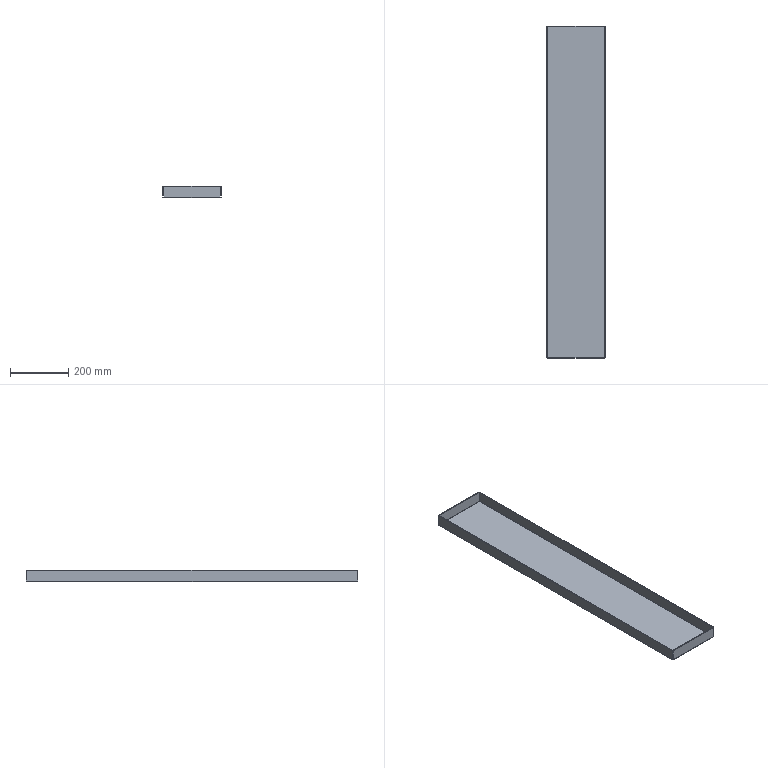Part | SolidWorks | features EdgeFlange 1, FlatPattern 1, SMBaseFlange 1, SheetMetal 1 | 1 solid | 38 faces | box 200 x 1140 x 40 mm | volume 654012 mm3 | plane 22 | spline 8 | cylinder 8 | commonest cylinder face diameters 1.473 x4 5.473 x4
STEP:
#1=CARTESIAN_POINT('',(97.263,567.263,-2.));
#2=VERTEX_POINT('',#1);
#3=CARTESIAN_POINT('',(97.263,-567.263,-2.));
#4=VERTEX_POINT('',#3);
#5=CARTESIAN_POINT('',(97.263,567.293,-2.));
#6=DIRECTION('',(0.,-1.,0.));
#7=VECTOR('',#6,1000.);
#8=LINE('',#5,#7);
#9=EDGE_CURVE('',#2,#4,#8,.T.);
#10=ORIENTED_EDGE('',*,*,#9,.T.);
#11=CARTESIAN_POINT('',(-97.263,-567.263,-2.));
#12=VERTEX_POINT('',#11);
#13=CARTESIAN_POINT('',(97.293,-567.263,-2.));
#14=DIRECTION('',(-1.,0.,0.));
#15=VECTOR('',#14,1000.);
#16=LINE('',#13,#15);
#17=EDGE_CURVE('',#4,#12,#16,.T.);
#18=ORIENTED_EDGE('',*,*,#17,.T.);
#19=CARTESIAN_POINT('',(-97.263,567.263,-2.));
#20=VERTEX_POINT('',#19);
#21=CARTESIAN_POINT('',(-97.263,-567.293,-2.));
#22=DIRECTION('',(0.,1.,0.));
#23=VECTOR('',#22,1000.);
#24=LINE('',#21,#23);
#25=EDGE_CURVE('',#12,#20,#24,.T.);
#26=ORIENTED_EDGE('',*,*,#25,.T.);
#27=CARTESIAN_POINT('',(-97.293,567.263,-2.));
#28=DIRECTION('',(1.,0.,0.));
#29=VECTOR('',#28,1000.);
#30=LINE('',#27,#29);
#31=EDGE_CURVE('',#20,#2,#30,.T.);
#32=ORIENTED_EDGE('',*,*,#31,.T.);
#33=EDGE_LOOP('',(#10,#18,#26,#32));
#34=FACE_OUTER_BOUND('',#33,.T.);
#35=CARTESIAN_POINT('',(0.,0.,-2.));
#36=DIRECTION('',(0.,0.,-1.));
#37=DIRECTION('',(-1.,0.,0.));
#38=AXIS2_PLACEMENT_3D('',#35,#36,#37);
#39=PLANE('',#38);
#40=ADVANCED_FACE('',(#34),#39,.T.);
#41=CARTESIAN_POINT('',(97.263,-567.263,0.));
#42=VERTEX_POINT('',#41);
#43=CARTESIAN_POINT('',(-97.263,-567.263,0.));
#44=VERTEX_POINT('',#43);
#45=CARTESIAN_POINT('',(97.293,-567.263,0.));
#46=DIRECTION('',(-1.,0.,0.));
#47=VECTOR('',#46,1000.);
#48=LINE('',#45,#47);
#49=EDGE_CURVE('',#42,#44,#48,.T.);
#50=ORIENTED_EDGE('',*,*,#49,.F.);
#51=CARTESIAN_POINT('',(97.263,567.263,0.));
#52=VERTEX_POINT('',#51);
#53=CARTESIAN_POINT('',(97.263,567.293,0.));
#54=DIRECTION('',(0.,-1.,0.));
#55=VECTOR('',#54,1000.);
#56=LINE('',#53,#55);
#57=EDGE_CURVE('',#52,#42,#56,.T.);
#58=ORIENTED_EDGE('',*,*,#57,.F.);
#59=CARTESIAN_POINT('',(-97.263,567.263,0.));
#60=VERTEX_POINT('',#59);
#61=CARTESIAN_POINT('',(-97.293,567.263,0.));
#62=DIRECTION('',(1.,0.,0.));
#63=VECTOR('',#62,1000.);
#64=LINE('',#61,#63);
#65=EDGE_CURVE('',#60,#52,#64,.T.);
#66=ORIENTED_EDGE('',*,*,#65,.F.);
#67=CARTESIAN_POINT('',(-97.263,-567.293,0.));
#68=DIRECTION('',(0.,1.,0.));
#69=VECTOR('',#68,1000.);
#70=LINE('',#67,#69);
#71=EDGE_CURVE('',#44,#60,#70,.T.);
#72=ORIENTED_EDGE('',*,*,#71,.F.);
#73=EDGE_LOOP('',(#50,#58,#66,#72));
#74=FACE_OUTER_BOUND('',#73,.T.);
#75=CARTESIAN_POINT('',(0.,0.,0.));
#76=DIRECTION('',(0.,0.,-1.));
#77=DIRECTION('',(-1.,0.,0.));
#78=AXIS2_PLACEMENT_3D('',#75,#76,#77);
#79=PLANE('',#78);
#80=ADVANCED_FACE('',(#74),#79,.F.);
#81=CARTESIAN_POINT('',(97.293,570.,0.7366));
#82=VERTEX_POINT('',#81);
#83=CARTESIAN_POINT('',(97.293,568.,0.7366));
#84=VERTEX_POINT('',#83);
#85=CARTESIAN_POINT('',(97.293,568.,0.7366));
#86=DIRECTION('',(0.,-1.,0.));
#87=VECTOR('',#86,1000.);
#88=LINE('',#85,#87);
#89=EDGE_CURVE('',#82,#84,#88,.T.);
#90=ORIENTED_EDGE('',*,*,#89,.T.);
#91=CARTESIAN_POINT('',(97.263,567.263,0.));
#92=CARTESIAN_POINT('',(97.268,567.456,0.));
#93=CARTESIAN_POINT('',(97.273,567.648,0.07939));
#94=CARTESIAN_POINT('',(97.283,567.921,0.3521));
#95=CARTESIAN_POINT('',(97.288,568.,0.5438));
#96=CARTESIAN_POINT('',(97.293,568.,0.7366));
#97=B_SPLINE_CURVE_WITH_KNOTS('',3,(#91,#92,#93,#94,#95,#96),.UNSPECIFIED.,.F.,.F.,(4,2,4),(0.,0.5,1.),.UNSPECIFIED.);
#98=EDGE_CURVE('',#52,#84,#97,.T.);
#99=ORIENTED_EDGE('',*,*,#98,.F.);
#100=CARTESIAN_POINT('',(97.263,567.263,0.));
#101=DIRECTION('',(0.,0.,-1.));
#102=VECTOR('',#101,1000.);
#103=LINE('',#100,#102);
#104=EDGE_CURVE('',#52,#2,#103,.T.);
#105=ORIENTED_EDGE('',*,*,#104,.T.);
#106=CARTESIAN_POINT('',(97.263,567.263,-2.));
#107=CARTESIAN_POINT('',(97.266,567.622,-2.));
#108=CARTESIAN_POINT('',(97.268,567.98,-1.929));
#109=CARTESIAN_POINT('',(97.273,568.642,-1.655));
#110=CARTESIAN_POINT('',(97.276,568.945,-1.452));
#111=CARTESIAN_POINT('',(97.281,569.452,-0.9452));
#112=CARTESIAN_POINT('',(97.283,569.655,-0.6416));
#113=CARTESIAN_POINT('',(97.288,569.929,0.0203));
#114=CARTESIAN_POINT('',(97.29,570.,0.3784));
#115=CARTESIAN_POINT('',(97.293,570.,0.7366));
#116=B_SPLINE_CURVE_WITH_KNOTS('',3,(#106,#107,#108,#109,#110,#111,#112,#113,#114,#115),.UNSPECIFIED.,.F.,.F.,(4,2,2,2,4),(0.,0.25,0.5,0.75,1.),.UNSPECIFIED.);
#117=EDGE_CURVE('',#2,#82,#116,.T.);
#118=ORIENTED_EDGE('',*,*,#117,.T.);
#119=EDGE_LOOP('',(#90,#99,#105,#118));
#120=FACE_OUTER_BOUND('',#119,.T.);
#121=CARTESIAN_POINT('',(97.263,567.263,-2.02));
#122=CARTESIAN_POINT('',(97.266,567.624,-2.02));
#123=CARTESIAN_POINT('',(97.268,567.985,-1.948));
#124=CARTESIAN_POINT('',(97.273,568.652,-1.672));
#125=CARTESIAN_POINT('',(97.276,568.957,-1.468));
#126=CARTESIAN_POINT('',(97.281,569.468,-0.9575));
#127=CARTESIAN_POINT('',(97.283,569.672,-0.6517));
#128=CARTESIAN_POINT('',(97.288,569.948,0.01507));
#129=CARTESIAN_POINT('',(97.29,570.02,0.3757));
#130=CARTESIAN_POINT('',(97.293,570.02,0.7366));
#131=CARTESIAN_POINT('',(97.263,567.263,-2.));
#132=CARTESIAN_POINT('',(97.266,567.622,-2.));
#133=CARTESIAN_POINT('',(97.268,567.98,-1.929));
#134=CARTESIAN_POINT('',(97.273,568.642,-1.655));
#135=CARTESIAN_POINT('',(97.276,568.945,-1.452));
#136=CARTESIAN_POINT('',(97.281,569.452,-0.9452));
#137=CARTESIAN_POINT('',(97.283,569.655,-0.6416));
#138=CARTESIAN_POINT('',(97.288,569.929,0.0203));
#139=CARTESIAN_POINT('',(97.29,570.,0.3783));
#140=CARTESIAN_POINT('',(97.293,570.,0.7366));
#141=CARTESIAN_POINT('',(97.263,567.263,0.));
#142=CARTESIAN_POINT('',(97.266,567.36,0.));
#143=CARTESIAN_POINT('',(97.268,567.456,0.01917));
#144=CARTESIAN_POINT('',(97.273,567.634,0.09297));
#145=CARTESIAN_POINT('',(97.276,567.716,0.1476));
#146=CARTESIAN_POINT('',(97.281,567.852,0.2839));
#147=CARTESIAN_POINT('',(97.283,567.907,0.3656));
#148=CARTESIAN_POINT('',(97.288,567.981,0.5438));
#149=CARTESIAN_POINT('',(97.29,568.,0.6402));
#150=CARTESIAN_POINT('',(97.293,568.,0.7366));
#151=CARTESIAN_POINT('',(97.263,567.263,0.0202));
#152=CARTESIAN_POINT('',(97.266,567.357,0.0202));
#153=CARTESIAN_POINT('',(97.268,567.451,0.03885));
#154=CARTESIAN_POINT('',(97.273,567.624,0.1106));
#155=CARTESIAN_POINT('',(97.276,567.704,0.1637));
#156=CARTESIAN_POINT('',(97.281,567.836,0.2963));
#157=CARTESIAN_POINT('',(97.283,567.889,0.3758));
#158=CARTESIAN_POINT('',(97.288,567.961,0.5491));
#159=CARTESIAN_POINT('',(97.29,567.98,0.6428));
#160=CARTESIAN_POINT('',(97.293,567.98,0.7366));
#161=B_SPLINE_SURFACE_WITH_KNOTS('',1,3,((#121,#122,#123,#124,#125,#126,#127,#128,#129,#130),(#131,#132,#133,#134,#135,#136,#137,#138,#139,#140),(#141,#142,#143,#144,#145,#146,#147,#148,#149,#150),(#151,#152,#153,#154,#155,#156,#157,#158,#159,#160)),.UNSPECIFIED.,.F.,.F.,.F.,(2,1,1,2),(4,2,2,2,4),(-0.01,0.,1.,1.01),(0.,0.25,0.5,0.75,1.),.UNSPECIFIED.);
#162=ADVANCED_FACE('',(#120),#161,.F.);
#163=CARTESIAN_POINT('',(-97.293,568.,0.7366));
#164=VERTEX_POINT('',#163);
#165=CARTESIAN_POINT('',(-97.293,568.,0.7366));
#166=CARTESIAN_POINT('',(-97.288,568.,0.5438));
#167=CARTESIAN_POINT('',(-97.283,567.921,0.3521));
#168=CARTESIAN_POINT('',(-97.273,567.648,0.07939));
#169=CARTESIAN_POINT('',(-97.268,567.456,0.));
#170=CARTESIAN_POINT('',(-97.263,567.263,0.));
#171=B_SPLINE_CURVE_WITH_KNOTS('',3,(#165,#166,#167,#168,#169,#170),.UNSPECIFIED.,.F.,.F.,(4,2,4),(0.,0.5,1.),.UNSPECIFIED.);
#172=EDGE_CURVE('',#164,#60,#171,.T.);
#173=ORIENTED_EDGE('',*,*,#172,.F.);
#174=CARTESIAN_POINT('',(-97.293,570.,0.7366));
#175=VERTEX_POINT('',#174);
#176=CARTESIAN_POINT('',(-97.293,568.,0.7366));
#177=DIRECTION('',(0.,-1.,0.));
#178=VECTOR('',#177,1000.);
#179=LINE('',#176,#178);
#180=EDGE_CURVE('',#175,#164,#179,.T.);
#181=ORIENTED_EDGE('',*,*,#180,.F.);
#182=CARTESIAN_POINT('',(-97.293,570.,0.7366));
#183=CARTESIAN_POINT('',(-97.29,570.,0.3784));
#184=CARTESIAN_POINT('',(-97.288,569.929,0.0203));
#185=CARTESIAN_POINT('',(-97.283,569.655,-0.6416));
#186=CARTESIAN_POINT('',(-97.281,569.452,-0.9452));
#187=CARTESIAN_POINT('',(-97.276,568.945,-1.452));
#188=CARTESIAN_POINT('',(-97.273,568.642,-1.655));
#189=CARTESIAN_POINT('',(-97.268,567.98,-1.929));
#190=CARTESIAN_POINT('',(-97.266,567.622,-2.));
#191=CARTESIAN_POINT('',(-97.263,567.263,-2.));
#192=B_SPLINE_CURVE_WITH_KNOTS('',3,(#182,#183,#184,#185,#186,#187,#188,#189,#190,#191),.UNSPECIFIED.,.F.,.F.,(4,2,2,2,4),(0.,0.25,0.5,0.75,1.),.UNSPECIFIED.);
#193=EDGE_CURVE('',#175,#20,#192,.T.);
#194=ORIENTED_EDGE('',*,*,#193,.T.);
#195=CARTESIAN_POINT('',(-97.263,567.263,0.));
#196=DIRECTION('',(0.,0.,-1.));
#197=VECTOR('',#196,1000.);
#198=LINE('',#195,#197);
#199=EDGE_CURVE('',#60,#20,#198,.T.);
#200=ORIENTED_EDGE('',*,*,#199,.F.);
#201=EDGE_LOOP('',(#173,#181,#194,#200));
#202=FACE_OUTER_BOUND('',#201,.T.);
#203=CARTESIAN_POINT('',(-97.293,570.02,0.7366));
#204=CARTESIAN_POINT('',(-97.29,570.02,0.3757));
#205=CARTESIAN_POINT('',(-97.288,569.948,0.01507));
#206=CARTESIAN_POINT('',(-97.283,569.672,-0.6517));
#207=CARTESIAN_POINT('',(-97.281,569.468,-0.9575));
#208=CARTESIAN_POINT('',(-97.276,568.957,-1.468));
#209=CARTESIAN_POINT('',(-97.273,568.652,-1.672));
#210=CARTESIAN_POINT('',(-97.268,567.985,-1.948));
#211=CARTESIAN_POINT('',(-97.266,567.624,-2.02));
#212=CARTESIAN_POINT('',(-97.263,567.263,-2.02));
#213=CARTESIAN_POINT('',(-97.293,570.,0.7366));
#214=CARTESIAN_POINT('',(-97.29,570.,0.3783));
#215=CARTESIAN_POINT('',(-97.288,569.929,0.0203));
#216=CARTESIAN_POINT('',(-97.283,569.655,-0.6416));
#217=CARTESIAN_POINT('',(-97.281,569.452,-0.9452));
#218=CARTESIAN_POINT('',(-97.276,568.945,-1.452));
#219=CARTESIAN_POINT('',(-97.273,568.642,-1.655));
#220=CARTESIAN_POINT('',(-97.268,567.98,-1.929));
#221=CARTESIAN_POINT('',(-97.266,567.622,-2.));
#222=CARTESIAN_POINT('',(-97.263,567.263,-2.));
#223=CARTESIAN_POINT('',(-97.293,568.,0.7366));
#224=CARTESIAN_POINT('',(-97.29,568.,0.6402));
#225=CARTESIAN_POINT('',(-97.288,567.981,0.5438));
#226=CARTESIAN_POINT('',(-97.283,567.907,0.3656));
#227=CARTESIAN_POINT('',(-97.281,567.852,0.2839));
#228=CARTESIAN_POINT('',(-97.276,567.716,0.1476));
#229=CARTESIAN_POINT('',(-97.273,567.634,0.09297));
#230=CARTESIAN_POINT('',(-97.268,567.456,0.01917));
#231=CARTESIAN_POINT('',(-97.266,567.36,0.));
#232=CARTESIAN_POINT('',(-97.263,567.263,0.));
#233=CARTESIAN_POINT('',(-97.293,567.98,0.7366));
#234=CARTESIAN_POINT('',(-97.29,567.98,0.6428));
#235=CARTESIAN_POINT('',(-97.288,567.961,0.5491));
#236=CARTESIAN_POINT('',(-97.283,567.889,0.3758));
#237=CARTESIAN_POINT('',(-97.281,567.836,0.2963));
#238=CARTESIAN_POINT('',(-97.276,567.704,0.1637));
#239=CARTESIAN_POINT('',(-97.273,567.624,0.1106));
#240=CARTESIAN_POINT('',(-97.268,567.451,0.03885));
#241=CARTESIAN_POINT('',(-97.266,567.357,0.0202));
#242=CARTESIAN_POINT('',(-97.263,567.263,0.0202));
#243=B_SPLINE_SURFACE_WITH_KNOTS('',1,3,((#203,#204,#205,#206,#207,#208,#209,#210,#211,#212),(#213,#214,#215,#216,#217,#218,#219,#220,#221,#222),(#223,#224,#225,#226,#227,#228,#229,#230,#231,#232),(#233,#234,#235,#236,#237,#238,#239,#240,#241,#242)),.UNSPECIFIED.,.F.,.F.,.F.,(2,1,1,2),(4,2,2,2,4),(-0.01,0.,1.,1.01),(0.,0.25,0.5,0.75,1.),.UNSPECIFIED.);
#244=ADVANCED_FACE('',(#202),#243,.F.);
#245=ORIENTED_EDGE('',*,*,#31,.F.);
#246=ORIENTED_EDGE('',*,*,#193,.F.);
#247=CARTESIAN_POINT('',(0.,570.,0.7366));
#248=DIRECTION('',(-1.,0.,0.));
#249=VECTOR('',#248,1000.);
#250=LINE('',#247,#249);
#251=EDGE_CURVE('',#82,#175,#250,.T.);
#252=ORIENTED_EDGE('',*,*,#251,.F.);
#253=ORIENTED_EDGE('',*,*,#117,.F.);
#254=EDGE_LOOP('',(#245,#246,#252,#253));
#255=FACE_OUTER_BOUND('',#254,.T.);
#256=CARTESIAN_POINT('',(-97.293,567.263,0.7366));
#257=DIRECTION('',(-1.,0.,0.));
#258=DIRECTION('',(0.,1.,0.));
#259=AXIS2_PLACEMENT_3D('',#256,#257,#258);
#260=CYLINDRICAL_SURFACE('',#259,2.737);
#261=ADVANCED_FACE('',(#255),#260,.T.);
#262=ORIENTED_EDGE('',*,*,#65,.T.);
#263=ORIENTED_EDGE('',*,*,#98,.T.);
#264=CARTESIAN_POINT('',(100.,568.,0.7366));
#265=DIRECTION('',(-1.,0.,0.));
#266=VECTOR('',#265,1000.);
#267=LINE('',#264,#266);
#268=EDGE_CURVE('',#84,#164,#267,.T.);
#269=ORIENTED_EDGE('',*,*,#268,.T.);
#270=ORIENTED_EDGE('',*,*,#172,.T.);
#271=EDGE_LOOP('',(#262,#263,#269,#270));
#272=FACE_OUTER_BOUND('',#271,.T.);
#273=CARTESIAN_POINT('',(-97.293,567.263,0.7366));
#274=DIRECTION('',(-1.,0.,0.));
#275=DIRECTION('',(0.,1.,0.));
#276=AXIS2_PLACEMENT_3D('',#273,#274,#275);
#277=CYLINDRICAL_SURFACE('',#276,0.7366);
#278=ADVANCED_FACE('',(#272),#277,.F.);
#279=CARTESIAN_POINT('',(97.293,568.,38.));
#280=VERTEX_POINT('',#279);
#281=CARTESIAN_POINT('',(97.293,570.,38.));
#282=VERTEX_POINT('',#281);
#283=CARTESIAN_POINT('',(97.293,570.,38.));
#284=DIRECTION('',(0.,1.,0.));
#285=VECTOR('',#284,1000.);
#286=LINE('',#283,#285);
#287=EDGE_CURVE('',#280,#282,#286,.T.);
#288=ORIENTED_EDGE('',*,*,#287,.F.);
#289=CARTESIAN_POINT('',(97.293,568.,0.));
#290=DIRECTION('',(0.,0.,1.));
#291=VECTOR('',#290,1000.);
#292=LINE('',#289,#291);
#293=EDGE_CURVE('',#84,#280,#292,.T.);
#294=ORIENTED_EDGE('',*,*,#293,.F.);
#295=ORIENTED_EDGE('',*,*,#89,.F.);
#296=CARTESIAN_POINT('',(97.293,570.,0.));
#297=DIRECTION('',(0.,0.,-1.));
#298=VECTOR('',#297,1000.);
#299=LINE('',#296,#298);
#300=EDGE_CURVE('',#282,#82,#299,.T.);
#301=ORIENTED_EDGE('',*,*,#300,.F.);
#302=EDGE_LOOP('',(#288,#294,#295,#301));
#303=FACE_OUTER_BOUND('',#302,.T.);
#304=CARTESIAN_POINT('',(97.293,568.,0.));
#305=DIRECTION('',(1.,0.,0.));
#306=DIRECTION('',(0.,0.,-1.));
#307=AXIS2_PLACEMENT_3D('',#304,#305,#306);
#308=PLANE('',#307);
#309=ADVANCED_FACE('',(#303),#308,.T.);
#310=CARTESIAN_POINT('',(-97.293,570.,38.));
#311=VERTEX_POINT('',#310);
#312=CARTESIAN_POINT('',(-97.293,570.,0.));
#313=DIRECTION('',(0.,0.,-1.));
#314=VECTOR('',#313,1000.);
#315=LINE('',#312,#314);
#316=EDGE_CURVE('',#311,#175,#315,.T.);
#317=ORIENTED_EDGE('',*,*,#316,.F.);
#318=CARTESIAN_POINT('',(-100.,570.,38.));
#319=DIRECTION('',(-1.,0.,0.));
#320=VECTOR('',#319,1000.);
#321=LINE('',#318,#320);
#322=EDGE_CURVE('',#282,#311,#321,.T.);
#323=ORIENTED_EDGE('',*,*,#322,.F.);
#324=ORIENTED_EDGE('',*,*,#300,.T.);
#325=ORIENTED_EDGE('',*,*,#251,.T.);
#326=EDGE_LOOP('',(#317,#323,#324,#325));
#327=FACE_OUTER_BOUND('',#326,.T.);
#328=CARTESIAN_POINT('',(0.,570.,0.));
#329=DIRECTION('',(0.,1.,0.));
#330=DIRECTION('',(0.,0.,1.));
#331=AXIS2_PLACEMENT_3D('',#328,#329,#330);
#332=PLANE('',#331);
#333=ADVANCED_FACE('',(#327),#332,.T.);
#334=CARTESIAN_POINT('',(-97.293,568.,38.));
#335=VERTEX_POINT('',#334);
#336=CARTESIAN_POINT('',(0.,568.,38.));
#337=DIRECTION('',(-1.,0.,0.));
#338=VECTOR('',#337,1000.);
#339=LINE('',#336,#338);
#340=EDGE_CURVE('',#280,#335,#339,.T.);
#341=ORIENTED_EDGE('',*,*,#340,.T.);
#342=CARTESIAN_POINT('',(-97.293,568.,0.));
#343=DIRECTION('',(0.,0.,1.));
#344=VECTOR('',#343,1000.);
#345=LINE('',#342,#344);
#346=EDGE_CURVE('',#164,#335,#345,.T.);
#347=ORIENTED_EDGE('',*,*,#346,.F.);
#348=ORIENTED_EDGE('',*,*,#268,.F.);
#349=ORIENTED_EDGE('',*,*,#293,.T.);
#350=EDGE_LOOP('',(#341,#347,#348,#349));
#351=FACE_OUTER_BOUND('',#350,.T.);
#352=CARTESIAN_POINT('',(0.,568.,0.));
#353=DIRECTION('',(0.,1.,0.));
#354=DIRECTION('',(0.,0.,1.));
#355=AXIS2_PLACEMENT_3D('',#352,#353,#354);
#356=PLANE('',#355);
#357=ADVANCED_FACE('',(#351),#356,.F.);
#358=CARTESIAN_POINT('',(-97.293,568.,38.));
#359=DIRECTION('',(0.,1.,0.));
#360=VECTOR('',#359,1000.);
#361=LINE('',#358,#360);
#362=EDGE_CURVE('',#335,#311,#361,.T.);
#363=ORIENTED_EDGE('',*,*,#362,.F.);
#364=ORIENTED_EDGE('',*,*,#340,.F.);
#365=ORIENTED_EDGE('',*,*,#287,.T.);
#366=ORIENTED_EDGE('',*,*,#322,.T.);
#367=EDGE_LOOP('',(#363,#364,#365,#366));
#368=FACE_OUTER_BOUND('',#367,.T.);
#369=CARTESIAN_POINT('',(-100.,570.,38.));
#370=DIRECTION('',(0.,0.,1.));
#371=DIRECTION('',(0.,-1.,0.));
#372=AXIS2_PLACEMENT_3D('',#369,#370,#371);
#373=PLANE('',#372);
#374=ADVANCED_FACE('',(#368),#373,.T.);
#375=ORIENTED_EDGE('',*,*,#346,.T.);
#376=ORIENTED_EDGE('',*,*,#362,.T.);
#377=ORIENTED_EDGE('',*,*,#316,.T.);
#378=ORIENTED_EDGE('',*,*,#180,.T.);
#379=EDGE_LOOP('',(#375,#376,#377,#378));
#380=FACE_OUTER_BOUND('',#379,.T.);
#381=CARTESIAN_POINT('',(-97.293,568.,0.));
#382=DIRECTION('',(1.,0.,0.));
#383=DIRECTION('',(0.,0.,-1.));
#384=AXIS2_PLACEMENT_3D('',#381,#382,#383);
#385=PLANE('',#384);
#386=ADVANCED_FACE('',(#380),#385,.F.);
#387=CARTESIAN_POINT('',(-100.,567.293,0.7366));
#388=VERTEX_POINT('',#387);
#389=CARTESIAN_POINT('',(-98.,567.293,0.7366));
#390=VERTEX_POINT('',#389);
#391=CARTESIAN_POINT('',(-98.,567.293,0.7366));
#392=DIRECTION('',(1.,0.,0.));
#393=VECTOR('',#392,1000.);
#394=LINE('',#391,#393);
#395=EDGE_CURVE('',#388,#390,#394,.T.);
#396=ORIENTED_EDGE('',*,*,#395,.T.);
#397=CARTESIAN_POINT('',(-97.263,567.263,0.));
#398=CARTESIAN_POINT('',(-97.456,567.268,0.));
#399=CARTESIAN_POINT('',(-97.648,567.273,0.07939));
#400=CARTESIAN_POINT('',(-97.921,567.283,0.3521));
#401=CARTESIAN_POINT('',(-98.,567.288,0.5438));
#402=CARTESIAN_POINT('',(-98.,567.293,0.7366));
#403=B_SPLINE_CURVE_WITH_KNOTS('',3,(#397,#398,#399,#400,#401,#402),.UNSPECIFIED.,.F.,.F.,(4,2,4),(0.,0.5,1.),.UNSPECIFIED.);
#404=EDGE_CURVE('',#60,#390,#403,.T.);
#405=ORIENTED_EDGE('',*,*,#404,.F.);
#406=ORIENTED_EDGE('',*,*,#199,.T.);
#407=CARTESIAN_POINT('',(-97.263,567.263,-2.));
#408=CARTESIAN_POINT('',(-97.622,567.266,-2.));
#409=CARTESIAN_POINT('',(-97.98,567.268,-1.929));
#410=CARTESIAN_POINT('',(-98.642,567.273,-1.655));
#411=CARTESIAN_POINT('',(-98.945,567.276,-1.452));
#412=CARTESIAN_POINT('',(-99.452,567.281,-0.9452));
#413=CARTESIAN_POINT('',(-99.655,567.283,-0.6416));
#414=CARTESIAN_POINT('',(-99.929,567.288,0.0203));
#415=CARTESIAN_POINT('',(-100.,567.29,0.3784));
#416=CARTESIAN_POINT('',(-100.,567.293,0.7366));
#417=B_SPLINE_CURVE_WITH_KNOTS('',3,(#407,#408,#409,#410,#411,#412,#413,#414,#415,#416),.UNSPECIFIED.,.F.,.F.,(4,2,2,2,4),(0.,0.25,0.5,0.75,1.),.UNSPECIFIED.);
#418=EDGE_CURVE('',#20,#388,#417,.T.);
#419=ORIENTED_EDGE('',*,*,#418,.T.);
#420=EDGE_LOOP('',(#396,#405,#406,#419));
#421=FACE_OUTER_BOUND('',#420,.T.);
#422=CARTESIAN_POINT('',(-97.263,567.263,-2.02));
#423=CARTESIAN_POINT('',(-97.624,567.266,-2.02));
#424=CARTESIAN_POINT('',(-97.985,567.268,-1.948));
#425=CARTESIAN_POINT('',(-98.652,567.273,-1.672));
#426=CARTESIAN_POINT('',(-98.957,567.276,-1.468));
#427=CARTESIAN_POINT('',(-99.468,567.281,-0.9575));
#428=CARTESIAN_POINT('',(-99.672,567.283,-0.6517));
#429=CARTESIAN_POINT('',(-99.948,567.288,0.01507));
#430=CARTESIAN_POINT('',(-100.02,567.29,0.3757));
#431=CARTESIAN_POINT('',(-100.02,567.293,0.7366));
#432=CARTESIAN_POINT('',(-97.263,567.263,-2.));
#433=CARTESIAN_POINT('',(-97.622,567.266,-2.));
#434=CARTESIAN_POINT('',(-97.98,567.268,-1.929));
#435=CARTESIAN_POINT('',(-98.642,567.273,-1.655));
#436=CARTESIAN_POINT('',(-98.945,567.276,-1.452));
#437=CARTESIAN_POINT('',(-99.452,567.281,-0.9452));
#438=CARTESIAN_POINT('',(-99.655,567.283,-0.6416));
#439=CARTESIAN_POINT('',(-99.929,567.288,0.0203));
#440=CARTESIAN_POINT('',(-100.,567.29,0.3783));
#441=CARTESIAN_POINT('',(-100.,567.293,0.7366));
#442=CARTESIAN_POINT('',(-97.263,567.263,0.));
#443=CARTESIAN_POINT('',(-97.36,567.266,0.));
#444=CARTESIAN_POINT('',(-97.456,567.268,0.01917));
#445=CARTESIAN_POINT('',(-97.634,567.273,0.09297));
#446=CARTESIAN_POINT('',(-97.716,567.276,0.1476));
#447=CARTESIAN_POINT('',(-97.852,567.281,0.2839));
#448=CARTESIAN_POINT('',(-97.907,567.283,0.3656));
#449=CARTESIAN_POINT('',(-97.981,567.288,0.5438));
#450=CARTESIAN_POINT('',(-98.,567.29,0.6402));
#451=CARTESIAN_POINT('',(-98.,567.293,0.7366));
#452=CARTESIAN_POINT('',(-97.263,567.263,0.0202));
#453=CARTESIAN_POINT('',(-97.357,567.266,0.0202));
#454=CARTESIAN_POINT('',(-97.451,567.268,0.03885));
#455=CARTESIAN_POINT('',(-97.624,567.273,0.1106));
#456=CARTESIAN_POINT('',(-97.704,567.276,0.1637));
#457=CARTESIAN_POINT('',(-97.836,567.281,0.2963));
#458=CARTESIAN_POINT('',(-97.889,567.283,0.3758));
#459=CARTESIAN_POINT('',(-97.961,567.288,0.5491));
#460=CARTESIAN_POINT('',(-97.98,567.29,0.6428));
#461=CARTESIAN_POINT('',(-97.98,567.293,0.7366));
#462=B_SPLINE_SURFACE_WITH_KNOTS('',1,3,((#422,#423,#424,#425,#426,#427,#428,#429,#430,#431),(#432,#433,#434,#435,#436,#437,#438,#439,#440,#441),(#442,#443,#444,#445,#446,#447,#448,#449,#450,#451),(#452,#453,#454,#455,#456,#457,#458,#459,#460,#461)),.UNSPECIFIED.,.F.,.F.,.F.,(2,1,1,2),(4,2,2,2,4),(-0.01,0.,1.,1.01),(0.,0.25,0.5,0.75,1.),.UNSPECIFIED.);
#463=ADVANCED_FACE('',(#421),#462,.F.);
#464=CARTESIAN_POINT('',(-98.,-567.293,0.7366));
#465=VERTEX_POINT('',#464);
#466=CARTESIAN_POINT('',(-98.,-567.293,0.7366));
#467=CARTESIAN_POINT('',(-98.,-567.288,0.5438));
#468=CARTESIAN_POINT('',(-97.921,-567.283,0.3521));
#469=CARTESIAN_POINT('',(-97.648,-567.273,0.07939));
#470=CARTESIAN_POINT('',(-97.456,-567.268,0.));
#471=CARTESIAN_POINT('',(-97.263,-567.263,0.));
#472=B_SPLINE_CURVE_WITH_KNOTS('',3,(#466,#467,#468,#469,#470,#471),.UNSPECIFIED.,.F.,.F.,(4,2,4),(0.,0.5,1.),.UNSPECIFIED.);
#473=EDGE_CURVE('',#465,#44,#472,.T.);
#474=ORIENTED_EDGE('',*,*,#473,.F.);
#475=CARTESIAN_POINT('',(-100.,-567.293,0.7366));
#476=VERTEX_POINT('',#475);
#477=CARTESIAN_POINT('',(-98.,-567.293,0.7366));
#478=DIRECTION('',(1.,0.,0.));
#479=VECTOR('',#478,1000.);
#480=LINE('',#477,#479);
#481=EDGE_CURVE('',#476,#465,#480,.T.);
#482=ORIENTED_EDGE('',*,*,#481,.F.);
#483=CARTESIAN_POINT('',(-100.,-567.293,0.7366));
#484=CARTESIAN_POINT('',(-100.,-567.29,0.3784));
#485=CARTESIAN_POINT('',(-99.929,-567.288,0.0203));
#486=CARTESIAN_POINT('',(-99.655,-567.283,-0.6416));
#487=CARTESIAN_POINT('',(-99.452,-567.281,-0.9452));
#488=CARTESIAN_POINT('',(-98.945,-567.276,-1.452));
#489=CARTESIAN_POINT('',(-98.642,-567.273,-1.655));
#490=CARTESIAN_POINT('',(-97.98,-567.268,-1.929));
#491=CARTESIAN_POINT('',(-97.622,-567.266,-2.));
#492=CARTESIAN_POINT('',(-97.263,-567.263,-2.));
#493=B_SPLINE_CURVE_WITH_KNOTS('',3,(#483,#484,#485,#486,#487,#488,#489,#490,#491,#492),.UNSPECIFIED.,.F.,.F.,(4,2,2,2,4),(0.,0.25,0.5,0.75,1.),.UNSPECIFIED.);
#494=EDGE_CURVE('',#476,#12,#493,.T.);
#495=ORIENTED_EDGE('',*,*,#494,.T.);
#496=CARTESIAN_POINT('',(-97.263,-567.263,0.));
#497=DIRECTION('',(0.,0.,-1.));
#498=VECTOR('',#497,1000.);
#499=LINE('',#496,#498);
#500=EDGE_CURVE('',#44,#12,#499,.T.);
#501=ORIENTED_EDGE('',*,*,#500,.F.);
#502=EDGE_LOOP('',(#474,#482,#495,#501));
#503=FACE_OUTER_BOUND('',#502,.T.);
#504=CARTESIAN_POINT('',(-100.02,-567.293,0.7366));
#505=CARTESIAN_POINT('',(-100.02,-567.29,0.3757));
#506=CARTESIAN_POINT('',(-99.948,-567.288,0.01507));
#507=CARTESIAN_POINT('',(-99.672,-567.283,-0.6517));
#508=CARTESIAN_POINT('',(-99.468,-567.281,-0.9575));
#509=CARTESIAN_POINT('',(-98.957,-567.276,-1.468));
#510=CARTESIAN_POINT('',(-98.652,-567.273,-1.672));
#511=CARTESIAN_POINT('',(-97.985,-567.268,-1.948));
#512=CARTESIAN_POINT('',(-97.624,-567.266,-2.02));
#513=CARTESIAN_POINT('',(-97.263,-567.263,-2.02));
#514=CARTESIAN_POINT('',(-100.,-567.293,0.7366));
#515=CARTESIAN_POINT('',(-100.,-567.29,0.3783));
#516=CARTESIAN_POINT('',(-99.929,-567.288,0.0203));
#517=CARTESIAN_POINT('',(-99.655,-567.283,-0.6416));
#518=CARTESIAN_POINT('',(-99.452,-567.281,-0.9452));
#519=CARTESIAN_POINT('',(-98.945,-567.276,-1.452));
#520=CARTESIAN_POINT('',(-98.642,-567.273,-1.655));
#521=CARTESIAN_POINT('',(-97.98,-567.268,-1.929));
#522=CARTESIAN_POINT('',(-97.622,-567.266,-2.));
#523=CARTESIAN_POINT('',(-97.263,-567.263,-2.));
#524=CARTESIAN_POINT('',(-98.,-567.293,0.7366));
#525=CARTESIAN_POINT('',(-98.,-567.29,0.6402));
#526=CARTESIAN_POINT('',(-97.981,-567.288,0.5438));
#527=CARTESIAN_POINT('',(-97.907,-567.283,0.3656));
#528=CARTESIAN_POINT('',(-97.852,-567.281,0.2839));
#529=CARTESIAN_POINT('',(-97.716,-567.276,0.1476));
#530=CARTESIAN_POINT('',(-97.634,-567.273,0.09297));
#531=CARTESIAN_POINT('',(-97.456,-567.268,0.01917));
#532=CARTESIAN_POINT('',(-97.36,-567.266,0.));
#533=CARTESIAN_POINT('',(-97.263,-567.263,0.));
#534=CARTESIAN_POINT('',(-97.98,-567.293,0.7366));
#535=CARTESIAN_POINT('',(-97.98,-567.29,0.6428));
#536=CARTESIAN_POINT('',(-97.961,-567.288,0.5491));
#537=CARTESIAN_POINT('',(-97.889,-567.283,0.3758));
#538=CARTESIAN_POINT('',(-97.836,-567.281,0.2963));
#539=CARTESIAN_POINT('',(-97.704,-567.276,0.1637));
#540=CARTESIAN_POINT('',(-97.624,-567.273,0.1106));
#541=CARTESIAN_POINT('',(-97.451,-567.268,0.03885));
#542=CARTESIAN_POINT('',(-97.357,-567.266,0.0202));
#543=CARTESIAN_POINT('',(-97.263,-567.263,0.0202));
#544=B_SPLINE_SURFACE_WITH_KNOTS('',1,3,((#504,#505,#506,#507,#508,#509,#510,#511,#512,#513),(#514,#515,#516,#517,#518,#519,#520,#521,#522,#523),(#524,#525,#526,#527,#528,#529,#530,#531,#532,#533),(#534,#535,#536,#537,#538,#539,#540,#541,#542,#543)),.UNSPECIFIED.,.F.,.F.,.F.,(2,1,1,2),(4,2,2,2,4),(-0.01,0.,1.,1.01),(0.,0.25,0.5,0.75,1.),.UNSPECIFIED.);
#545=ADVANCED_FACE('',(#503),#544,.F.);
#546=ORIENTED_EDGE('',*,*,#25,.F.);
#547=ORIENTED_EDGE('',*,*,#494,.F.);
#548=CARTESIAN_POINT('',(-100.,570.,0.7366));
#549=DIRECTION('',(0.,1.,0.));
#550=VECTOR('',#549,1000.);
#551=LINE('',#548,#550);
#552=EDGE_CURVE('',#476,#388,#551,.T.);
#553=ORIENTED_EDGE('',*,*,#552,.T.);
#554=ORIENTED_EDGE('',*,*,#418,.F.);
#555=EDGE_LOOP('',(#546,#547,#553,#554));
#556=FACE_OUTER_BOUND('',#555,.T.);
#557=CARTESIAN_POINT('',(-97.263,-567.293,0.7366));
#558=DIRECTION('',(0.,-1.,0.));
#559=DIRECTION('',(-1.,0.,0.));
#560=AXIS2_PLACEMENT_3D('',#557,#558,#559);
#561=CYLINDRICAL_SURFACE('',#560,2.737);
#562=ADVANCED_FACE('',(#556),#561,.T.);
#563=ORIENTED_EDGE('',*,*,#71,.T.);
#564=ORIENTED_EDGE('',*,*,#404,.T.);
#565=CARTESIAN_POINT('',(-98.,570.,0.7366));
#566=DIRECTION('',(0.,-1.,0.));
#567=VECTOR('',#566,1000.);
#568=LINE('',#565,#567);
#569=EDGE_CURVE('',#390,#465,#568,.T.);
#570=ORIENTED_EDGE('',*,*,#569,.T.);
#571=ORIENTED_EDGE('',*,*,#473,.T.);
#572=EDGE_LOOP('',(#563,#564,#570,#571));
#573=FACE_OUTER_BOUND('',#572,.T.);
#574=CARTESIAN_POINT('',(-97.263,-567.293,0.7366));
#575=DIRECTION('',(0.,-1.,0.));
#576=DIRECTION('',(-1.,0.,0.));
#577=AXIS2_PLACEMENT_3D('',#574,#575,#576);
#578=CYLINDRICAL_SURFACE('',#577,0.7366);
#579=ADVANCED_FACE('',(#573),#578,.F.);
#580=CARTESIAN_POINT('',(-98.,567.293,38.));
#581=VERTEX_POINT('',#580);
#582=CARTESIAN_POINT('',(-100.,567.293,38.));
#583=VERTEX_POINT('',#582);
#584=CARTESIAN_POINT('',(-100.,567.293,38.));
#585=DIRECTION('',(-1.,0.,0.));
#586=VECTOR('',#585,1000.);
#587=LINE('',#584,#586);
#588=EDGE_CURVE('',#581,#583,#587,.T.);
#589=ORIENTED_EDGE('',*,*,#588,.F.);
#590=CARTESIAN_POINT('',(-98.,567.293,0.));
#591=DIRECTION('',(0.,0.,1.));
#592=VECTOR('',#591,1000.);
#593=LINE('',#590,#592);
#594=EDGE_CURVE('',#390,#581,#593,.T.);
#595=ORIENTED_EDGE('',*,*,#594,.F.);
#596=ORIENTED_EDGE('',*,*,#395,.F.);
#597=CARTESIAN_POINT('',(-100.,567.293,0.));
#598=DIRECTION('',(0.,0.,1.));
#599=VECTOR('',#598,1000.);
#600=LINE('',#597,#599);
#601=EDGE_CURVE('',#388,#583,#600,.T.);
#602=ORIENTED_EDGE('',*,*,#601,.T.);
#603=EDGE_LOOP('',(#589,#595,#596,#602));
#604=FACE_OUTER_BOUND('',#603,.T.);
#605=CARTESIAN_POINT('',(-98.,567.293,0.));
#606=DIRECTION('',(0.,1.,0.));
#607=DIRECTION('',(0.,0.,1.));
#608=AXIS2_PLACEMENT_3D('',#605,#606,#607);
#609=PLANE('',#608);
#610=ADVANCED_FACE('',(#604),#609,.T.);
#611=ORIENTED_EDGE('',*,*,#552,.F.);
#612=CARTESIAN_POINT('',(-100.,-567.293,38.));
#613=VERTEX_POINT('',#612);
#614=CARTESIAN_POINT('',(-100.,-567.293,0.));
#615=DIRECTION('',(0.,0.,1.));
#616=VECTOR('',#615,1000.);
#617=LINE('',#614,#616);
#618=EDGE_CURVE('',#476,#613,#617,.T.);
#619=ORIENTED_EDGE('',*,*,#618,.T.);
#620=CARTESIAN_POINT('',(-100.,570.,38.));
#621=DIRECTION('',(0.,-1.,0.));
#622=VECTOR('',#621,1000.);
#623=LINE('',#620,#622);
#624=EDGE_CURVE('',#583,#613,#623,.T.);
#625=ORIENTED_EDGE('',*,*,#624,.F.);
#626=ORIENTED_EDGE('',*,*,#601,.F.);
#627=EDGE_LOOP('',(#611,#619,#625,#626));
#628=FACE_OUTER_BOUND('',#627,.T.);
#629=CARTESIAN_POINT('',(-100.,0.,0.));
#630=DIRECTION('',(1.,0.,0.));
#631=DIRECTION('',(0.,0.,-1.));
#632=AXIS2_PLACEMENT_3D('',#629,#630,#631);
#633=PLANE('',#632);
#634=ADVANCED_FACE('',(#628),#633,.F.);
#635=CARTESIAN_POINT('',(-98.,-567.293,38.));
#636=VERTEX_POINT('',#635);
#637=CARTESIAN_POINT('',(-98.,-567.293,0.));
#638=DIRECTION('',(0.,0.,1.));
#639=VECTOR('',#638,1000.);
#640=LINE('',#637,#639);
#641=EDGE_CURVE('',#465,#636,#640,.T.);
#642=ORIENTED_EDGE('',*,*,#641,.F.);
#643=ORIENTED_EDGE('',*,*,#569,.F.);
#644=ORIENTED_EDGE('',*,*,#594,.T.);
#645=CARTESIAN_POINT('',(-98.,0.,38.));
#646=DIRECTION('',(0.,-1.,0.));
#647=VECTOR('',#646,1000.);
#648=LINE('',#645,#647);
#649=EDGE_CURVE('',#581,#636,#648,.T.);
#650=ORIENTED_EDGE('',*,*,#649,.T.);
#651=EDGE_LOOP('',(#642,#643,#644,#650));
#652=FACE_OUTER_BOUND('',#651,.T.);
#653=CARTESIAN_POINT('',(-98.,0.,0.));
#654=DIRECTION('',(1.,0.,0.));
#655=DIRECTION('',(0.,0.,-1.));
#656=AXIS2_PLACEMENT_3D('',#653,#654,#655);
#657=PLANE('',#656);
#658=ADVANCED_FACE('',(#652),#657,.T.);
#659=CARTESIAN_POINT('',(-98.,-567.293,38.));
#660=DIRECTION('',(-1.,0.,0.));
#661=VECTOR('',#660,1000.);
#662=LINE('',#659,#661);
#663=EDGE_CURVE('',#636,#613,#662,.T.);
#664=ORIENTED_EDGE('',*,*,#663,.F.);
#665=ORIENTED_EDGE('',*,*,#649,.F.);
#666=ORIENTED_EDGE('',*,*,#588,.T.);
#667=ORIENTED_EDGE('',*,*,#624,.T.);
#668=EDGE_LOOP('',(#664,#665,#666,#667));
#669=FACE_OUTER_BOUND('',#668,.T.);
#670=CARTESIAN_POINT('',(-100.,570.,38.));
#671=DIRECTION('',(0.,0.,1.));
#672=DIRECTION('',(1.,0.,0.));
#673=AXIS2_PLACEMENT_3D('',#670,#671,#672);
#674=PLANE('',#673);
#675=ADVANCED_FACE('',(#669),#674,.T.);
#676=ORIENTED_EDGE('',*,*,#641,.T.);
#677=ORIENTED_EDGE('',*,*,#663,.T.);
#678=ORIENTED_EDGE('',*,*,#618,.F.);
#679=ORIENTED_EDGE('',*,*,#481,.T.);
#680=EDGE_LOOP('',(#676,#677,#678,#679));
#681=FACE_OUTER_BOUND('',#680,.T.);
#682=CARTESIAN_POINT('',(-98.,-567.293,0.));
#683=DIRECTION('',(0.,1.,0.));
#684=DIRECTION('',(0.,0.,1.));
#685=AXIS2_PLACEMENT_3D('',#682,#683,#684);
#686=PLANE('',#685);
#687=ADVANCED_FACE('',(#681),#686,.F.);
#688=CARTESIAN_POINT('',(100.,-567.293,0.7366));
#689=VERTEX_POINT('',#688);
#690=CARTESIAN_POINT('',(98.,-567.293,0.7366));
#691=VERTEX_POINT('',#690);
#692=CARTESIAN_POINT('',(98.,-567.293,0.7366));
#693=DIRECTION('',(-1.,0.,0.));
#694=VECTOR('',#693,1000.);
#695=LINE('',#692,#694);
#696=EDGE_CURVE('',#689,#691,#695,.T.);
#697=ORIENTED_EDGE('',*,*,#696,.T.);
#698=CARTESIAN_POINT('',(97.263,-567.263,0.));
#699=CARTESIAN_POINT('',(97.456,-567.268,0.));
#700=CARTESIAN_POINT('',(97.648,-567.273,0.07939));
#701=CARTESIAN_POINT('',(97.921,-567.283,0.3521));
#702=CARTESIAN_POINT('',(98.,-567.288,0.5438));
#703=CARTESIAN_POINT('',(98.,-567.293,0.7366));
#704=B_SPLINE_CURVE_WITH_KNOTS('',3,(#698,#699,#700,#701,#702,#703),.UNSPECIFIED.,.F.,.F.,(4,2,4),(0.,0.5,1.),.UNSPECIFIED.);
#705=EDGE_CURVE('',#42,#691,#704,.T.);
#706=ORIENTED_EDGE('',*,*,#705,.F.);
#707=CARTESIAN_POINT('',(97.263,-567.263,0.));
#708=DIRECTION('',(0.,0.,-1.));
#709=VECTOR('',#708,1000.);
#710=LINE('',#707,#709);
#711=EDGE_CURVE('',#42,#4,#710,.T.);
#712=ORIENTED_EDGE('',*,*,#711,.T.);
#713=CARTESIAN_POINT('',(97.263,-567.263,-2.));
#714=CARTESIAN_POINT('',(97.622,-567.266,-2.));
#715=CARTESIAN_POINT('',(97.98,-567.268,-1.929));
#716=CARTESIAN_POINT('',(98.642,-567.273,-1.655));
#717=CARTESIAN_POINT('',(98.945,-567.276,-1.452));
#718=CARTESIAN_POINT('',(99.452,-567.281,-0.9452));
#719=CARTESIAN_POINT('',(99.655,-567.283,-0.6416));
#720=CARTESIAN_POINT('',(99.929,-567.288,0.0203));
#721=CARTESIAN_POINT('',(100.,-567.29,0.3784));
#722=CARTESIAN_POINT('',(100.,-567.293,0.7366));
#723=B_SPLINE_CURVE_WITH_KNOTS('',3,(#713,#714,#715,#716,#717,#718,#719,#720,#721,#722),.UNSPECIFIED.,.F.,.F.,(4,2,2,2,4),(0.,0.25,0.5,0.75,1.),.UNSPECIFIED.);
#724=EDGE_CURVE('',#4,#689,#723,.T.);
#725=ORIENTED_EDGE('',*,*,#724,.T.);
#726=EDGE_LOOP('',(#697,#706,#712,#725));
#727=FACE_OUTER_BOUND('',#726,.T.);
#728=CARTESIAN_POINT('',(97.263,-567.263,-2.02));
#729=CARTESIAN_POINT('',(97.624,-567.266,-2.02));
#730=CARTESIAN_POINT('',(97.985,-567.268,-1.948));
#731=CARTESIAN_POINT('',(98.652,-567.273,-1.672));
#732=CARTESIAN_POINT('',(98.957,-567.276,-1.468));
#733=CARTESIAN_POINT('',(99.468,-567.281,-0.9575));
#734=CARTESIAN_POINT('',(99.672,-567.283,-0.6517));
#735=CARTESIAN_POINT('',(99.948,-567.288,0.01507));
#736=CARTESIAN_POINT('',(100.02,-567.29,0.3757));
#737=CARTESIAN_POINT('',(100.02,-567.293,0.7366));
#738=CARTESIAN_POINT('',(97.263,-567.263,-2.));
#739=CARTESIAN_POINT('',(97.622,-567.266,-2.));
#740=CARTESIAN_POINT('',(97.98,-567.268,-1.929));
#741=CARTESIAN_POINT('',(98.642,-567.273,-1.655));
#742=CARTESIAN_POINT('',(98.945,-567.276,-1.452));
#743=CARTESIAN_POINT('',(99.452,-567.281,-0.9452));
#744=CARTESIAN_POINT('',(99.655,-567.283,-0.6416));
#745=CARTESIAN_POINT('',(99.929,-567.288,0.0203));
#746=CARTESIAN_POINT('',(100.,-567.29,0.3783));
#747=CARTESIAN_POINT('',(100.,-567.293,0.7366));
#748=CARTESIAN_POINT('',(97.263,-567.263,0.));
#749=CARTESIAN_POINT('',(97.36,-567.266,0.));
#750=CARTESIAN_POINT('',(97.456,-567.268,0.01917));
#751=CARTESIAN_POINT('',(97.634,-567.273,0.09297));
#752=CARTESIAN_POINT('',(97.716,-567.276,0.1476));
#753=CARTESIAN_POINT('',(97.852,-567.281,0.2839));
#754=CARTESIAN_POINT('',(97.907,-567.283,0.3656));
#755=CARTESIAN_POINT('',(97.981,-567.288,0.5438));
#756=CARTESIAN_POINT('',(98.,-567.29,0.6402));
#757=CARTESIAN_POINT('',(98.,-567.293,0.7366));
#758=CARTESIAN_POINT('',(97.263,-567.263,0.0202));
#759=CARTESIAN_POINT('',(97.357,-567.266,0.0202));
#760=CARTESIAN_POINT('',(97.451,-567.268,0.03885));
#761=CARTESIAN_POINT('',(97.624,-567.273,0.1106));
#762=CARTESIAN_POINT('',(97.704,-567.276,0.1637));
#763=CARTESIAN_POINT('',(97.836,-567.281,0.2963));
#764=CARTESIAN_POINT('',(97.889,-567.283,0.3758));
#765=CARTESIAN_POINT('',(97.961,-567.288,0.5491));
#766=CARTESIAN_POINT('',(97.98,-567.29,0.6428));
#767=CARTESIAN_POINT('',(97.98,-567.293,0.7366));
#768=B_SPLINE_SURFACE_WITH_KNOTS('',1,3,((#728,#729,#730,#731,#732,#733,#734,#735,#736,#737),(#738,#739,#740,#741,#742,#743,#744,#745,#746,#747),(#748,#749,#750,#751,#752,#753,#754,#755,#756,#757),(#758,#759,#760,#761,#762,#763,#764,#765,#766,#767)),.UNSPECIFIED.,.F.,.F.,.F.,(2,1,1,2),(4,2,2,2,4),(-0.01,0.,1.,1.01),(0.,0.25,0.5,0.75,1.),.UNSPECIFIED.);
#769=ADVANCED_FACE('',(#727),#768,.F.);
#770=CARTESIAN_POINT('',(98.,567.293,0.7366));
#771=VERTEX_POINT('',#770);
#772=CARTESIAN_POINT('',(98.,567.293,0.7366));
#773=CARTESIAN_POINT('',(98.,567.288,0.5438));
#774=CARTESIAN_POINT('',(97.921,567.283,0.3521));
#775=CARTESIAN_POINT('',(97.648,567.273,0.07939));
#776=CARTESIAN_POINT('',(97.456,567.268,0.));
#777=CARTESIAN_POINT('',(97.263,567.263,0.));
#778=B_SPLINE_CURVE_WITH_KNOTS('',3,(#772,#773,#774,#775,#776,#777),.UNSPECIFIED.,.F.,.F.,(4,2,4),(0.,0.5,1.),.UNSPECIFIED.);
#779=EDGE_CURVE('',#771,#52,#778,.T.);
#780=ORIENTED_EDGE('',*,*,#779,.F.);
#781=CARTESIAN_POINT('',(100.,567.293,0.7366));
#782=VERTEX_POINT('',#781);
#783=CARTESIAN_POINT('',(98.,567.293,0.7366));
#784=DIRECTION('',(-1.,0.,0.));
#785=VECTOR('',#784,1000.);
#786=LINE('',#783,#785);
#787=EDGE_CURVE('',#782,#771,#786,.T.);
#788=ORIENTED_EDGE('',*,*,#787,.F.);
#789=CARTESIAN_POINT('',(100.,567.293,0.7366));
#790=CARTESIAN_POINT('',(100.,567.29,0.3784));
#791=CARTESIAN_POINT('',(99.929,567.288,0.0203));
#792=CARTESIAN_POINT('',(99.655,567.283,-0.6416));
#793=CARTESIAN_POINT('',(99.452,567.281,-0.9452));
#794=CARTESIAN_POINT('',(98.945,567.276,-1.452));
#795=CARTESIAN_POINT('',(98.642,567.273,-1.655));
#796=CARTESIAN_POINT('',(97.98,567.268,-1.929));
#797=CARTESIAN_POINT('',(97.622,567.266,-2.));
#798=CARTESIAN_POINT('',(97.263,567.263,-2.));
#799=B_SPLINE_CURVE_WITH_KNOTS('',3,(#789,#790,#791,#792,#793,#794,#795,#796,#797,#798),.UNSPECIFIED.,.F.,.F.,(4,2,2,2,4),(0.,0.25,0.5,0.75,1.),.UNSPECIFIED.);
#800=EDGE_CURVE('',#782,#2,#799,.T.);
#801=ORIENTED_EDGE('',*,*,#800,.T.);
#802=ORIENTED_EDGE('',*,*,#104,.F.);
#803=EDGE_LOOP('',(#780,#788,#801,#802));
#804=FACE_OUTER_BOUND('',#803,.T.);
#805=CARTESIAN_POINT('',(100.02,567.293,0.7366));
#806=CARTESIAN_POINT('',(100.02,567.29,0.3757));
#807=CARTESIAN_POINT('',(99.948,567.288,0.01507));
#808=CARTESIAN_POINT('',(99.672,567.283,-0.6517));
#809=CARTESIAN_POINT('',(99.468,567.281,-0.9575));
#810=CARTESIAN_POINT('',(98.957,567.276,-1.468));
#811=CARTESIAN_POINT('',(98.652,567.273,-1.672));
#812=CARTESIAN_POINT('',(97.985,567.268,-1.948));
#813=CARTESIAN_POINT('',(97.624,567.266,-2.02));
#814=CARTESIAN_POINT('',(97.263,567.263,-2.02));
#815=CARTESIAN_POINT('',(100.,567.293,0.7366));
#816=CARTESIAN_POINT('',(100.,567.29,0.3783));
#817=CARTESIAN_POINT('',(99.929,567.288,0.0203));
#818=CARTESIAN_POINT('',(99.655,567.283,-0.6416));
#819=CARTESIAN_POINT('',(99.452,567.281,-0.9452));
#820=CARTESIAN_POINT('',(98.945,567.276,-1.452));
#821=CARTESIAN_POINT('',(98.642,567.273,-1.655));
#822=CARTESIAN_POINT('',(97.98,567.268,-1.929));
#823=CARTESIAN_POINT('',(97.622,567.266,-2.));
#824=CARTESIAN_POINT('',(97.263,567.263,-2.));
#825=CARTESIAN_POINT('',(98.,567.293,0.7366));
#826=CARTESIAN_POINT('',(98.,567.29,0.6402));
#827=CARTESIAN_POINT('',(97.981,567.288,0.5438));
#828=CARTESIAN_POINT('',(97.907,567.283,0.3656));
#829=CARTESIAN_POINT('',(97.852,567.281,0.2839));
#830=CARTESIAN_POINT('',(97.716,567.276,0.1476));
#831=CARTESIAN_POINT('',(97.634,567.273,0.09297));
#832=CARTESIAN_POINT('',(97.456,567.268,0.01917));
#833=CARTESIAN_POINT('',(97.36,567.266,0.));
#834=CARTESIAN_POINT('',(97.263,567.263,0.));
#835=CARTESIAN_POINT('',(97.98,567.293,0.7366));
#836=CARTESIAN_POINT('',(97.98,567.29,0.6428));
#837=CARTESIAN_POINT('',(97.961,567.288,0.5491));
#838=CARTESIAN_POINT('',(97.889,567.283,0.3758));
#839=CARTESIAN_POINT('',(97.836,567.281,0.2963));
#840=CARTESIAN_POINT('',(97.704,567.276,0.1637));
#841=CARTESIAN_POINT('',(97.624,567.273,0.1106));
#842=CARTESIAN_POINT('',(97.451,567.268,0.03885));
#843=CARTESIAN_POINT('',(97.357,567.266,0.0202));
#844=CARTESIAN_POINT('',(97.263,567.263,0.0202));
#845=B_SPLINE_SURFACE_WITH_KNOTS('',1,3,((#805,#806,#807,#808,#809,#810,#811,#812,#813,#814),(#815,#816,#817,#818,#819,#820,#821,#822,#823,#824),(#825,#826,#827,#828,#829,#830,#831,#832,#833,#834),(#835,#836,#837,#838,#839,#840,#841,#842,#843,#844)),.UNSPECIFIED.,.F.,.F.,.F.,(2,1,1,2),(4,2,2,2,4),(-0.01,0.,1.,1.01),(0.,0.25,0.5,0.75,1.),.UNSPECIFIED.);
#846=ADVANCED_FACE('',(#804),#845,.F.);
#847=ORIENTED_EDGE('',*,*,#9,.F.);
#848=ORIENTED_EDGE('',*,*,#800,.F.);
#849=CARTESIAN_POINT('',(100.,-570.,0.7366));
#850=DIRECTION('',(0.,-1.,0.));
#851=VECTOR('',#850,1000.);
#852=LINE('',#849,#851);
#853=EDGE_CURVE('',#782,#689,#852,.T.);
#854=ORIENTED_EDGE('',*,*,#853,.T.);
#855=ORIENTED_EDGE('',*,*,#724,.F.);
#856=EDGE_LOOP('',(#847,#848,#854,#855));
#857=FACE_OUTER_BOUND('',#856,.T.);
#858=CARTESIAN_POINT('',(97.263,567.293,0.7366));
#859=DIRECTION('',(0.,1.,0.));
#860=DIRECTION('',(1.,0.,0.));
#861=AXIS2_PLACEMENT_3D('',#858,#859,#860);
#862=CYLINDRICAL_SURFACE('',#861,2.737);
#863=ADVANCED_FACE('',(#857),#862,.T.);
#864=ORIENTED_EDGE('',*,*,#57,.T.);
#865=ORIENTED_EDGE('',*,*,#705,.T.);
#866=CARTESIAN_POINT('',(98.,-570.,0.7366));
#867=DIRECTION('',(0.,1.,0.));
#868=VECTOR('',#867,1000.);
#869=LINE('',#866,#868);
#870=EDGE_CURVE('',#691,#771,#869,.T.);
#871=ORIENTED_EDGE('',*,*,#870,.T.);
#872=ORIENTED_EDGE('',*,*,#779,.T.);
#873=EDGE_LOOP('',(#864,#865,#871,#872));
#874=FACE_OUTER_BOUND('',#873,.T.);
#875=CARTESIAN_POINT('',(97.263,567.293,0.7366));
#876=DIRECTION('',(0.,1.,0.));
#877=DIRECTION('',(1.,0.,0.));
#878=AXIS2_PLACEMENT_3D('',#875,#876,#877);
#879=CYLINDRICAL_SURFACE('',#878,0.7366);
#880=ADVANCED_FACE('',(#874),#879,.F.);
#881=CARTESIAN_POINT('',(98.,-567.293,38.));
#882=VERTEX_POINT('',#881);
#883=CARTESIAN_POINT('',(100.,-567.293,38.));
#884=VERTEX_POINT('',#883);
#885=CARTESIAN_POINT('',(100.,-567.293,38.));
#886=DIRECTION('',(1.,0.,0.));
#887=VECTOR('',#886,1000.);
#888=LINE('',#885,#887);
#889=EDGE_CURVE('',#882,#884,#888,.T.);
#890=ORIENTED_EDGE('',*,*,#889,.F.);
#891=CARTESIAN_POINT('',(98.,-567.293,0.));
#892=DIRECTION('',(0.,0.,1.));
#893=VECTOR('',#892,1000.);
#894=LINE('',#891,#893);
#895=EDGE_CURVE('',#691,#882,#894,.T.);
#896=ORIENTED_EDGE('',*,*,#895,.F.);
#897=ORIENTED_EDGE('',*,*,#696,.F.);
#898=CARTESIAN_POINT('',(100.,-567.293,0.));
#899=DIRECTION('',(0.,0.,1.));
#900=VECTOR('',#899,1000.);
#901=LINE('',#898,#900);
#902=EDGE_CURVE('',#689,#884,#901,.T.);
#903=ORIENTED_EDGE('',*,*,#902,.T.);
#904=EDGE_LOOP('',(#890,#896,#897,#903));
#905=FACE_OUTER_BOUND('',#904,.T.);
#906=CARTESIAN_POINT('',(98.,-567.293,0.));
#907=DIRECTION('',(0.,-1.,0.));
#908=DIRECTION('',(0.,0.,-1.));
#909=AXIS2_PLACEMENT_3D('',#906,#907,#908);
#910=PLANE('',#909);
#911=ADVANCED_FACE('',(#905),#910,.T.);
#912=ORIENTED_EDGE('',*,*,#853,.F.);
#913=CARTESIAN_POINT('',(100.,567.293,38.));
#914=VERTEX_POINT('',#913);
#915=CARTESIAN_POINT('',(100.,567.293,0.));
#916=DIRECTION('',(0.,0.,1.));
#917=VECTOR('',#916,1000.);
#918=LINE('',#915,#917);
#919=EDGE_CURVE('',#782,#914,#918,.T.);
#920=ORIENTED_EDGE('',*,*,#919,.T.);
#921=CARTESIAN_POINT('',(100.,-570.,38.));
#922=DIRECTION('',(0.,1.,0.));
#923=VECTOR('',#922,1000.);
#924=LINE('',#921,#923);
#925=EDGE_CURVE('',#884,#914,#924,.T.);
#926=ORIENTED_EDGE('',*,*,#925,.F.);
#927=ORIENTED_EDGE('',*,*,#902,.F.);
#928=EDGE_LOOP('',(#912,#920,#926,#927));
#929=FACE_OUTER_BOUND('',#928,.T.);
#930=CARTESIAN_POINT('',(100.,0.,0.));
#931=DIRECTION('',(-1.,0.,0.));
#932=DIRECTION('',(0.,0.,1.));
#933=AXIS2_PLACEMENT_3D('',#930,#931,#932);
#934=PLANE('',#933);
#935=ADVANCED_FACE('',(#929),#934,.F.);
#936=CARTESIAN_POINT('',(98.,567.293,38.));
#937=VERTEX_POINT('',#936);
#938=CARTESIAN_POINT('',(98.,567.293,0.));
#939=DIRECTION('',(0.,0.,1.));
#940=VECTOR('',#939,1000.);
#941=LINE('',#938,#940);
#942=EDGE_CURVE('',#771,#937,#941,.T.);
#943=ORIENTED_EDGE('',*,*,#942,.F.);
#944=ORIENTED_EDGE('',*,*,#870,.F.);
#945=ORIENTED_EDGE('',*,*,#895,.T.);
#946=CARTESIAN_POINT('',(98.,0.,38.));
#947=DIRECTION('',(0.,1.,0.));
#948=VECTOR('',#947,1000.);
#949=LINE('',#946,#948);
#950=EDGE_CURVE('',#882,#937,#949,.T.);
#951=ORIENTED_EDGE('',*,*,#950,.T.);
#952=EDGE_LOOP('',(#943,#944,#945,#951));
#953=FACE_OUTER_BOUND('',#952,.T.);
#954=CARTESIAN_POINT('',(98.,0.,0.));
#955=DIRECTION('',(-1.,0.,0.));
#956=DIRECTION('',(0.,0.,1.));
#957=AXIS2_PLACEMENT_3D('',#954,#955,#956);
#958=PLANE('',#957);
#959=ADVANCED_FACE('',(#953),#958,.T.);
#960=CARTESIAN_POINT('',(98.,567.293,38.));
#961=DIRECTION('',(1.,0.,0.));
#962=VECTOR('',#961,1000.);
#963=LINE('',#960,#962);
#964=EDGE_CURVE('',#937,#914,#963,.T.);
#965=ORIENTED_EDGE('',*,*,#964,.F.);
#966=ORIENTED_EDGE('',*,*,#950,.F.);
#967=ORIENTED_EDGE('',*,*,#889,.T.);
#968=ORIENTED_EDGE('',*,*,#925,.T.);
#969=EDGE_LOOP('',(#965,#966,#967,#968));
#970=FACE_OUTER_BOUND('',#969,.T.);
#971=CARTESIAN_POINT('',(100.,-570.,38.));
#972=DIRECTION('',(0.,0.,1.));
#973=DIRECTION('',(1.,0.,0.));
#974=AXIS2_PLACEMENT_3D('',#971,#972,#973);
#975=PLANE('',#974);
#976=ADVANCED_FACE('',(#970),#975,.T.);
#977=ORIENTED_EDGE('',*,*,#942,.T.);
#978=ORIENTED_EDGE('',*,*,#964,.T.);
#979=ORIENTED_EDGE('',*,*,#919,.F.);
#980=ORIENTED_EDGE('',*,*,#787,.T.);
#981=EDGE_LOOP('',(#977,#978,#979,#980));
#982=FACE_OUTER_BOUND('',#981,.T.);
#983=CARTESIAN_POINT('',(98.,567.293,0.));
#984=DIRECTION('',(0.,-1.,0.));
#985=DIRECTION('',(0.,0.,-1.));
#986=AXIS2_PLACEMENT_3D('',#983,#984,#985);
#987=PLANE('',#986);
#988=ADVANCED_FACE('',(#982),#987,.F.);
#989=CARTESIAN_POINT('',(-97.293,-570.,0.7366));
#990=VERTEX_POINT('',#989);
#991=CARTESIAN_POINT('',(-97.293,-568.,0.7366));
#992=VERTEX_POINT('',#991);
#993=CARTESIAN_POINT('',(-97.293,-568.,0.7366));
#994=DIRECTION('',(0.,1.,0.));
#995=VECTOR('',#994,1000.);
#996=LINE('',#993,#995);
#997=EDGE_CURVE('',#990,#992,#996,.T.);
#998=ORIENTED_EDGE('',*,*,#997,.T.);
#999=CARTESIAN_POINT('',(-97.263,-567.263,0.));
#1000=CARTESIAN_POINT('',(-97.268,-567.456,0.));
#1001=CARTESIAN_POINT('',(-97.273,-567.648,0.07939));
#1002=CARTESIAN_POINT('',(-97.283,-567.921,0.3521));
#1003=CARTESIAN_POINT('',(-97.288,-568.,0.5438));
#1004=CARTESIAN_POINT('',(-97.293,-568.,0.7366));
#1005=B_SPLINE_CURVE_WITH_KNOTS('',3,(#999,#1000,#1001,#1002,#1003,#1004),.UNSPECIFIED.,.F.,.F.,(4,2,4),(0.,0.5,1.),.UNSPECIFIED.);
#1006=EDGE_CURVE('',#44,#992,#1005,.T.);
#1007=ORIENTED_EDGE('',*,*,#1006,.F.);
#1008=ORIENTED_EDGE('',*,*,#500,.T.);
#1009=CARTESIAN_POINT('',(-97.263,-567.263,-2.));
#1010=CARTESIAN_POINT('',(-97.266,-567.622,-2.));
#1011=CARTESIAN_POINT('',(-97.268,-567.98,-1.929));
#1012=CARTESIAN_POINT('',(-97.273,-568.642,-1.655));
#1013=CARTESIAN_POINT('',(-97.276,-568.945,-1.452));
#1014=CARTESIAN_POINT('',(-97.281,-569.452,-0.9452));
#1015=CARTESIAN_POINT('',(-97.283,-569.655,-0.6416));
#1016=CARTESIAN_POINT('',(-97.288,-569.929,0.0203));
#1017=CARTESIAN_POINT('',(-97.29,-570.,0.3784));
#1018=CARTESIAN_POINT('',(-97.293,-570.,0.7366));
#1019=B_SPLINE_CURVE_WITH_KNOTS('',3,(#1009,#1010,#1011,#1012,#1013,#1014,#1015,#1016,#1017,#1018),.UNSPECIFIED.,.F.,.F.,(4,2,2,2,4),(0.,0.25,0.5,0.75,1.),.UNSPECIFIED.);
#1020=EDGE_CURVE('',#12,#990,#1019,.T.);
#1021=ORIENTED_EDGE('',*,*,#1020,.T.);
#1022=EDGE_LOOP('',(#998,#1007,#1008,#1021));
#1023=FACE_OUTER_BOUND('',#1022,.T.);
#1024=CARTESIAN_POINT('',(-97.263,-567.263,-2.02));
#1025=CARTESIAN_POINT('',(-97.266,-567.624,-2.02));
#1026=CARTESIAN_POINT('',(-97.268,-567.985,-1.948));
#1027=CARTESIAN_POINT('',(-97.273,-568.652,-1.672));
#1028=CARTESIAN_POINT('',(-97.276,-568.957,-1.468));
#1029=CARTESIAN_POINT('',(-97.281,-569.468,-0.9575));
#1030=CARTESIAN_POINT('',(-97.283,-569.672,-0.6517));
#1031=CARTESIAN_POINT('',(-97.288,-569.948,0.01507));
#1032=CARTESIAN_POINT('',(-97.29,-570.02,0.3757));
#1033=CARTESIAN_POINT('',(-97.293,-570.02,0.7366));
#1034=CARTESIAN_POINT('',(-97.263,-567.263,-2.));
#1035=CARTESIAN_POINT('',(-97.266,-567.622,-2.));
#1036=CARTESIAN_POINT('',(-97.268,-567.98,-1.929));
#1037=CARTESIAN_POINT('',(-97.273,-568.642,-1.655));
#1038=CARTESIAN_POINT('',(-97.276,-568.945,-1.452));
#1039=CARTESIAN_POINT('',(-97.281,-569.452,-0.9452));
#1040=CARTESIAN_POINT('',(-97.283,-569.655,-0.6416));
#1041=CARTESIAN_POINT('',(-97.288,-569.929,0.0203));
#1042=CARTESIAN_POINT('',(-97.29,-570.,0.3783));
#1043=CARTESIAN_POINT('',(-97.293,-570.,0.7366));
#1044=CARTESIAN_POINT('',(-97.263,-567.263,0.));
#1045=CARTESIAN_POINT('',(-97.266,-567.36,0.));
#1046=CARTESIAN_POINT('',(-97.268,-567.456,0.01917));
#1047=CARTESIAN_POINT('',(-97.273,-567.634,0.09297));
#1048=CARTESIAN_POINT('',(-97.276,-567.716,0.1476));
#1049=CARTESIAN_POINT('',(-97.281,-567.852,0.2839));
#1050=CARTESIAN_POINT('',(-97.283,-567.907,0.3656));
#1051=CARTESIAN_POINT('',(-97.288,-567.981,0.5438));
#1052=CARTESIAN_POINT('',(-97.29,-568.,0.6402));
#1053=CARTESIAN_POINT('',(-97.293,-568.,0.7366));
#1054=CARTESIAN_POINT('',(-97.263,-567.263,0.0202));
#1055=CARTESIAN_POINT('',(-97.266,-567.357,0.0202));
#1056=CARTESIAN_POINT('',(-97.268,-567.451,0.03885));
#1057=CARTESIAN_POINT('',(-97.273,-567.624,0.1106));
#1058=CARTESIAN_POINT('',(-97.276,-567.704,0.1637));
#1059=CARTESIAN_POINT('',(-97.281,-567.836,0.2963));
#1060=CARTESIAN_POINT('',(-97.283,-567.889,0.3758));
#1061=CARTESIAN_POINT('',(-97.288,-567.961,0.5491));
#1062=CARTESIAN_POINT('',(-97.29,-567.98,0.6428));
#1063=CARTESIAN_POINT('',(-97.293,-567.98,0.7366));
#1064=B_SPLINE_SURFACE_WITH_KNOTS('',1,3,((#1024,#1025,#1026,#1027,#1028,#1029,#1030,#1031,#1032,#1033),(#1034,#1035,#1036,#1037,#1038,#1039,#1040,#1041,#1042,#1043),(#1044,#1045,#1046,#1047,#1048,#1049,#1050,#1051,#1052,#1053),(#1054,#1055,#1056,#1057,#1058,#1059,#1060,#1061,#1062,#1063)),.UNSPECIFIED.,.F.,.F.,.F.,(2,1,1,2),(4,2,2,2,4),(-0.01,0.,1.,1.01),(0.,0.25,0.5,0.75,1.),.UNSPECIFIED.);
#1065=ADVANCED_FACE('',(#1023),#1064,.F.);
#1066=CARTESIAN_POINT('',(97.293,-568.,0.7366));
#1067=VERTEX_POINT('',#1066);
#1068=CARTESIAN_POINT('',(97.293,-568.,0.7366));
#1069=CARTESIAN_POINT('',(97.288,-568.,0.5438));
#1070=CARTESIAN_POINT('',(97.283,-567.921,0.3521));
#1071=CARTESIAN_POINT('',(97.273,-567.648,0.07939));
#1072=CARTESIAN_POINT('',(97.268,-567.456,0.));
#1073=CARTESIAN_POINT('',(97.263,-567.263,0.));
#1074=B_SPLINE_CURVE_WITH_KNOTS('',3,(#1068,#1069,#1070,#1071,#1072,#1073),.UNSPECIFIED.,.F.,.F.,(4,2,4),(0.,0.5,1.),.UNSPECIFIED.);
#1075=EDGE_CURVE('',#1067,#42,#1074,.T.);
#1076=ORIENTED_EDGE('',*,*,#1075,.F.);
#1077=CARTESIAN_POINT('',(97.293,-570.,0.7366));
#1078=VERTEX_POINT('',#1077);
#1079=CARTESIAN_POINT('',(97.293,-568.,0.7366));
#1080=DIRECTION('',(0.,1.,0.));
#1081=VECTOR('',#1080,1000.);
#1082=LINE('',#1079,#1081);
#1083=EDGE_CURVE('',#1078,#1067,#1082,.T.);
#1084=ORIENTED_EDGE('',*,*,#1083,.F.);
#1085=CARTESIAN_POINT('',(97.293,-570.,0.7366));
#1086=CARTESIAN_POINT('',(97.29,-570.,0.3784));
#1087=CARTESIAN_POINT('',(97.288,-569.929,0.0203));
#1088=CARTESIAN_POINT('',(97.283,-569.655,-0.6416));
#1089=CARTESIAN_POINT('',(97.281,-569.452,-0.9452));
#1090=CARTESIAN_POINT('',(97.276,-568.945,-1.452));
#1091=CARTESIAN_POINT('',(97.273,-568.642,-1.655));
#1092=CARTESIAN_POINT('',(97.268,-567.98,-1.929));
#1093=CARTESIAN_POINT('',(97.266,-567.622,-2.));
#1094=CARTESIAN_POINT('',(97.263,-567.263,-2.));
#1095=B_SPLINE_CURVE_WITH_KNOTS('',3,(#1085,#1086,#1087,#1088,#1089,#1090,#1091,#1092,#1093,#1094),.UNSPECIFIED.,.F.,.F.,(4,2,2,2,4),(0.,0.25,0.5,0.75,1.),.UNSPECIFIED.);
#1096=EDGE_CURVE('',#1078,#4,#1095,.T.);
#1097=ORIENTED_EDGE('',*,*,#1096,.T.);
#1098=ORIENTED_EDGE('',*,*,#711,.F.);
#1099=EDGE_LOOP('',(#1076,#1084,#1097,#1098));
#1100=FACE_OUTER_BOUND('',#1099,.T.);
#1101=CARTESIAN_POINT('',(97.293,-570.02,0.7366));
#1102=CARTESIAN_POINT('',(97.29,-570.02,0.3757));
#1103=CARTESIAN_POINT('',(97.288,-569.948,0.01507));
#1104=CARTESIAN_POINT('',(97.283,-569.672,-0.6517));
#1105=CARTESIAN_POINT('',(97.281,-569.468,-0.9575));
#1106=CARTESIAN_POINT('',(97.276,-568.957,-1.468));
#1107=CARTESIAN_POINT('',(97.273,-568.652,-1.672));
#1108=CARTESIAN_POINT('',(97.268,-567.985,-1.948));
#1109=CARTESIAN_POINT('',(97.266,-567.624,-2.02));
#1110=CARTESIAN_POINT('',(97.263,-567.263,-2.02));
#1111=CARTESIAN_POINT('',(97.293,-570.,0.7366));
#1112=CARTESIAN_POINT('',(97.29,-570.,0.3783));
#1113=CARTESIAN_POINT('',(97.288,-569.929,0.0203));
#1114=CARTESIAN_POINT('',(97.283,-569.655,-0.6416));
#1115=CARTESIAN_POINT('',(97.281,-569.452,-0.9452));
#1116=CARTESIAN_POINT('',(97.276,-568.945,-1.452));
#1117=CARTESIAN_POINT('',(97.273,-568.642,-1.655));
#1118=CARTESIAN_POINT('',(97.268,-567.98,-1.929));
#1119=CARTESIAN_POINT('',(97.266,-567.622,-2.));
#1120=CARTESIAN_POINT('',(97.263,-567.263,-2.));
#1121=CARTESIAN_POINT('',(97.293,-568.,0.7366));
#1122=CARTESIAN_POINT('',(97.29,-568.,0.6402));
#1123=CARTESIAN_POINT('',(97.288,-567.981,0.5438));
#1124=CARTESIAN_POINT('',(97.283,-567.907,0.3656));
#1125=CARTESIAN_POINT('',(97.281,-567.852,0.2839));
#1126=CARTESIAN_POINT('',(97.276,-567.716,0.1476));
#1127=CARTESIAN_POINT('',(97.273,-567.634,0.09297));
#1128=CARTESIAN_POINT('',(97.268,-567.456,0.01917));
#1129=CARTESIAN_POINT('',(97.266,-567.36,0.));
#1130=CARTESIAN_POINT('',(97.263,-567.263,0.));
#1131=CARTESIAN_POINT('',(97.293,-567.98,0.7366));
#1132=CARTESIAN_POINT('',(97.29,-567.98,0.6428));
#1133=CARTESIAN_POINT('',(97.288,-567.961,0.5491));
#1134=CARTESIAN_POINT('',(97.283,-567.889,0.3758));
#1135=CARTESIAN_POINT('',(97.281,-567.836,0.2963));
#1136=CARTESIAN_POINT('',(97.276,-567.704,0.1637));
#1137=CARTESIAN_POINT('',(97.273,-567.624,0.1106));
#1138=CARTESIAN_POINT('',(97.268,-567.451,0.03885));
#1139=CARTESIAN_POINT('',(97.266,-567.357,0.0202));
#1140=CARTESIAN_POINT('',(97.263,-567.263,0.0202));
#1141=B_SPLINE_SURFACE_WITH_KNOTS('',1,3,((#1101,#1102,#1103,#1104,#1105,#1106,#1107,#1108,#1109,#1110),(#1111,#1112,#1113,#1114,#1115,#1116,#1117,#1118,#1119,#1120),(#1121,#1122,#1123,#1124,#1125,#1126,#1127,#1128,#1129,#1130),(#1131,#1132,#1133,#1134,#1135,#1136,#1137,#1138,#1139,#1140)),.UNSPECIFIED.,.F.,.F.,.F.,(2,1,1,2),(4,2,2,2,4),(-0.01,0.,1.,1.01),(0.,0.25,0.5,0.75,1.),.UNSPECIFIED.);
#1142=ADVANCED_FACE('',(#1100),#1141,.F.);
#1143=ORIENTED_EDGE('',*,*,#17,.F.);
#1144=ORIENTED_EDGE('',*,*,#1096,.F.);
#1145=CARTESIAN_POINT('',(-100.,-570.,0.7366));
#1146=DIRECTION('',(-1.,0.,0.));
#1147=VECTOR('',#1146,1000.);
#1148=LINE('',#1145,#1147);
#1149=EDGE_CURVE('',#1078,#990,#1148,.T.);
#1150=ORIENTED_EDGE('',*,*,#1149,.T.);
#1151=ORIENTED_EDGE('',*,*,#1020,.F.);
#1152=EDGE_LOOP('',(#1143,#1144,#1150,#1151));
#1153=FACE_OUTER_BOUND('',#1152,.T.);
#1154=CARTESIAN_POINT('',(97.293,-567.263,0.7366));
#1155=DIRECTION('',(1.,0.,0.));
#1156=DIRECTION('',(0.,-1.,0.));
#1157=AXIS2_PLACEMENT_3D('',#1154,#1155,#1156);
#1158=CYLINDRICAL_SURFACE('',#1157,2.737);
#1159=ADVANCED_FACE('',(#1153),#1158,.T.);
#1160=ORIENTED_EDGE('',*,*,#49,.T.);
#1161=ORIENTED_EDGE('',*,*,#1006,.T.);
#1162=CARTESIAN_POINT('',(-100.,-568.,0.7366));
#1163=DIRECTION('',(1.,0.,0.));
#1164=VECTOR('',#1163,1000.);
#1165=LINE('',#1162,#1164);
#1166=EDGE_CURVE('',#992,#1067,#1165,.T.);
#1167=ORIENTED_EDGE('',*,*,#1166,.T.);
#1168=ORIENTED_EDGE('',*,*,#1075,.T.);
#1169=EDGE_LOOP('',(#1160,#1161,#1167,#1168));
#1170=FACE_OUTER_BOUND('',#1169,.T.);
#1171=CARTESIAN_POINT('',(97.293,-567.263,0.7366));
#1172=DIRECTION('',(1.,0.,0.));
#1173=DIRECTION('',(0.,-1.,0.));
#1174=AXIS2_PLACEMENT_3D('',#1171,#1172,#1173);
#1175=CYLINDRICAL_SURFACE('',#1174,0.7366);
#1176=ADVANCED_FACE('',(#1170),#1175,.F.);
#1177=CARTESIAN_POINT('',(-97.293,-568.,38.));
#1178=VERTEX_POINT('',#1177);
#1179=CARTESIAN_POINT('',(-97.293,-570.,38.));
#1180=VERTEX_POINT('',#1179);
#1181=CARTESIAN_POINT('',(-97.293,-570.,38.));
#1182=DIRECTION('',(0.,-1.,0.));
#1183=VECTOR('',#1182,1000.);
#1184=LINE('',#1181,#1183);
#1185=EDGE_CURVE('',#1178,#1180,#1184,.T.);
#1186=ORIENTED_EDGE('',*,*,#1185,.F.);
#1187=CARTESIAN_POINT('',(-97.293,-568.,0.));
#1188=DIRECTION('',(0.,0.,1.));
#1189=VECTOR('',#1188,1000.);
#1190=LINE('',#1187,#1189);
#1191=EDGE_CURVE('',#992,#1178,#1190,.T.);
#1192=ORIENTED_EDGE('',*,*,#1191,.F.);
#1193=ORIENTED_EDGE('',*,*,#997,.F.);
#1194=CARTESIAN_POINT('',(-97.293,-570.,0.));
#1195=DIRECTION('',(0.,0.,1.));
#1196=VECTOR('',#1195,1000.);
#1197=LINE('',#1194,#1196);
#1198=EDGE_CURVE('',#990,#1180,#1197,.T.);
#1199=ORIENTED_EDGE('',*,*,#1198,.T.);
#1200=EDGE_LOOP('',(#1186,#1192,#1193,#1199));
#1201=FACE_OUTER_BOUND('',#1200,.T.);
#1202=CARTESIAN_POINT('',(-97.293,-568.,0.));
#1203=DIRECTION('',(-1.,0.,0.));
#1204=DIRECTION('',(0.,0.,1.));
#1205=AXIS2_PLACEMENT_3D('',#1202,#1203,#1204);
#1206=PLANE('',#1205);
#1207=ADVANCED_FACE('',(#1201),#1206,.T.);
#1208=ORIENTED_EDGE('',*,*,#1149,.F.);
#1209=CARTESIAN_POINT('',(97.293,-570.,38.));
#1210=VERTEX_POINT('',#1209);
#1211=CARTESIAN_POINT('',(97.293,-570.,0.));
#1212=DIRECTION('',(0.,0.,1.));
#1213=VECTOR('',#1212,1000.);
#1214=LINE('',#1211,#1213);
#1215=EDGE_CURVE('',#1078,#1210,#1214,.T.);
#1216=ORIENTED_EDGE('',*,*,#1215,.T.);
#1217=CARTESIAN_POINT('',(-100.,-570.,38.));
#1218=DIRECTION('',(1.,0.,0.));
#1219=VECTOR('',#1218,1000.);
#1220=LINE('',#1217,#1219);
#1221=EDGE_CURVE('',#1180,#1210,#1220,.T.);
#1222=ORIENTED_EDGE('',*,*,#1221,.F.);
#1223=ORIENTED_EDGE('',*,*,#1198,.F.);
#1224=EDGE_LOOP('',(#1208,#1216,#1222,#1223));
#1225=FACE_OUTER_BOUND('',#1224,.T.);
#1226=CARTESIAN_POINT('',(0.,-570.,0.));
#1227=DIRECTION('',(0.,1.,0.));
#1228=DIRECTION('',(0.,0.,1.));
#1229=AXIS2_PLACEMENT_3D('',#1226,#1227,#1228);
#1230=PLANE('',#1229);
#1231=ADVANCED_FACE('',(#1225),#1230,.F.);
#1232=CARTESIAN_POINT('',(97.293,-568.,38.));
#1233=VERTEX_POINT('',#1232);
#1234=CARTESIAN_POINT('',(97.293,-568.,0.));
#1235=DIRECTION('',(0.,0.,1.));
#1236=VECTOR('',#1235,1000.);
#1237=LINE('',#1234,#1236);
#1238=EDGE_CURVE('',#1067,#1233,#1237,.T.);
#1239=ORIENTED_EDGE('',*,*,#1238,.F.);
#1240=ORIENTED_EDGE('',*,*,#1166,.F.);
#1241=ORIENTED_EDGE('',*,*,#1191,.T.);
#1242=CARTESIAN_POINT('',(0.,-568.,38.));
#1243=DIRECTION('',(1.,0.,0.));
#1244=VECTOR('',#1243,1000.);
#1245=LINE('',#1242,#1244);
#1246=EDGE_CURVE('',#1178,#1233,#1245,.T.);
#1247=ORIENTED_EDGE('',*,*,#1246,.T.);
#1248=EDGE_LOOP('',(#1239,#1240,#1241,#1247));
#1249=FACE_OUTER_BOUND('',#1248,.T.);
#1250=CARTESIAN_POINT('',(0.,-568.,0.));
#1251=DIRECTION('',(0.,1.,0.));
#1252=DIRECTION('',(0.,0.,1.));
#1253=AXIS2_PLACEMENT_3D('',#1250,#1251,#1252);
#1254=PLANE('',#1253);
#1255=ADVANCED_FACE('',(#1249),#1254,.T.);
#1256=CARTESIAN_POINT('',(97.293,-568.,38.));
#1257=DIRECTION('',(0.,-1.,0.));
#1258=VECTOR('',#1257,1000.);
#1259=LINE('',#1256,#1258);
#1260=EDGE_CURVE('',#1233,#1210,#1259,.T.);
#1261=ORIENTED_EDGE('',*,*,#1260,.F.);
#1262=ORIENTED_EDGE('',*,*,#1246,.F.);
#1263=ORIENTED_EDGE('',*,*,#1185,.T.);
#1264=ORIENTED_EDGE('',*,*,#1221,.T.);
#1265=EDGE_LOOP('',(#1261,#1262,#1263,#1264));
#1266=FACE_OUTER_BOUND('',#1265,.T.);
#1267=CARTESIAN_POINT('',(-100.,-570.,38.));
#1268=DIRECTION('',(0.,0.,1.));
#1269=DIRECTION('',(0.,-1.,0.));
#1270=AXIS2_PLACEMENT_3D('',#1267,#1268,#1269);
#1271=PLANE('',#1270);
#1272=ADVANCED_FACE('',(#1266),#1271,.T.);
#1273=ORIENTED_EDGE('',*,*,#1238,.T.);
#1274=ORIENTED_EDGE('',*,*,#1260,.T.);
#1275=ORIENTED_EDGE('',*,*,#1215,.F.);
#1276=ORIENTED_EDGE('',*,*,#1083,.T.);
#1277=EDGE_LOOP('',(#1273,#1274,#1275,#1276));
#1278=FACE_OUTER_BOUND('',#1277,.T.);
#1279=CARTESIAN_POINT('',(97.293,-568.,0.));
#1280=DIRECTION('',(-1.,0.,0.));
#1281=DIRECTION('',(0.,0.,1.));
#1282=AXIS2_PLACEMENT_3D('',#1279,#1280,#1281);
#1283=PLANE('',#1282);
#1284=ADVANCED_FACE('',(#1278),#1283,.F.);
#1285=CLOSED_SHELL('',(#40,#80,#162,#244,#261,#278,#309,#333,#357,#374,#386,#463,#545,#562,#579,#610,#634,#658,#675,#687,#769,#846,#863,#880,#911,#935,#959,#976,#988,#1065,#1142,#1159,#1176,#1207,#1231,#1255,#1272,#1284));
#1286=MANIFOLD_SOLID_BREP('',#1285);
#1287=CARTESIAN_POINT('',(0.,0.,0.));
#1288=DIRECTION('',(0.,0.,1.));
#1289=DIRECTION('',(1.,0.,0.));
#1290=AXIS2_PLACEMENT_3D('',#1287,#1288,#1289);
#1291=(LENGTH_UNIT()NAMED_UNIT(*)SI_UNIT(.MILLI.,.METRE.));
#1292=UNCERTAINTY_MEASURE_WITH_UNIT(LENGTH_MEASURE(0.00001),#1291,'','');
#1293=(NAMED_UNIT(*)PLANE_ANGLE_UNIT()SI_UNIT($,.RADIAN.));
#1294=(NAMED_UNIT(*)SI_UNIT($,.STERADIAN.)SOLID_ANGLE_UNIT());
#1295=(GEOMETRIC_REPRESENTATION_CONTEXT(3)GLOBAL_UNCERTAINTY_ASSIGNED_CONTEXT((#1292))GLOBAL_UNIT_ASSIGNED_CONTEXT((#1291,#1293,#1294))REPRESENTATION_CONTEXT('',''));
#1296=ADVANCED_BREP_SHAPE_REPRESENTATION('',(#1286,#1290),#1295);